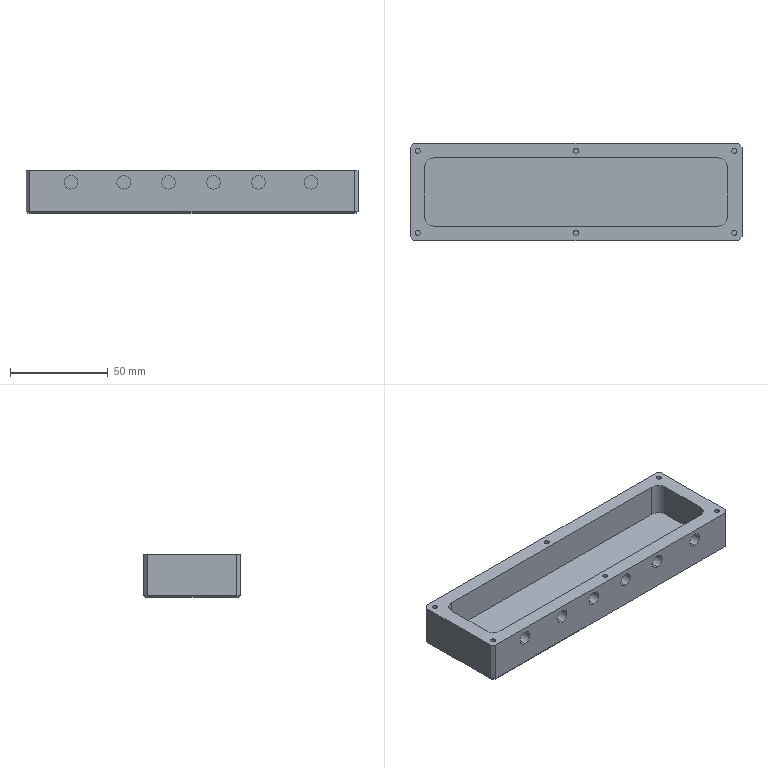Part | STEP file | Seal lower box | 1 solid | 57 faces | box 170 x 50 x 22 mm | volume 92795 mm3 | plane 29 | cylinder 28 | commonest cylinder face diameters 2.5 x12 7 x12 10 x4